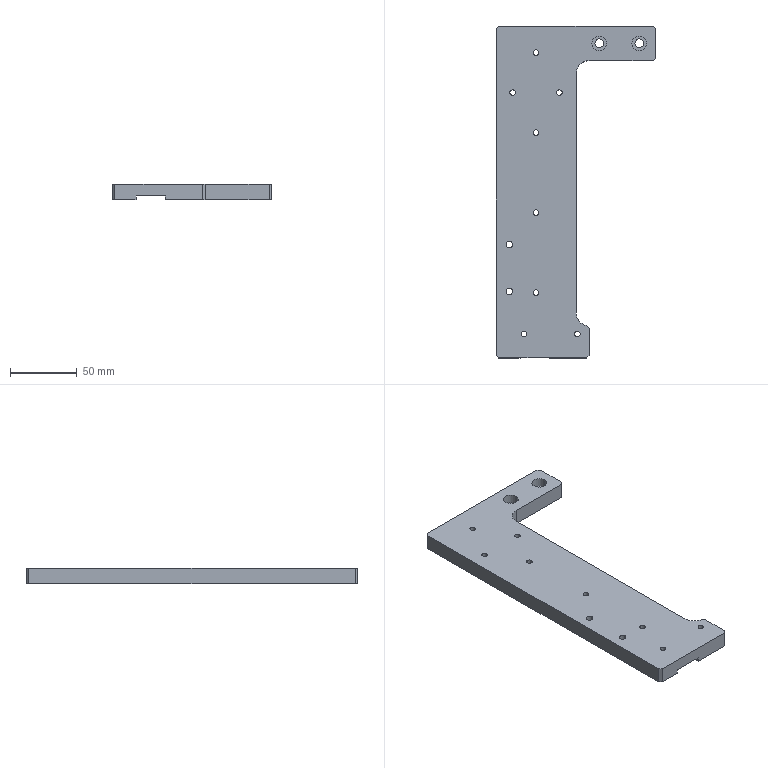Part | SolidWorks | features HoleWzd 5, Chamfer 1, Extrusion 1, ICE 1 | 1 solid | 51 faces | box 120 x 249 x 12 mm | volume 181549 mm3 | cylinder 30 | plane 21 | commonest cylinder face diameters 4.2 x16 5 x4 6.6 x4 11 x4 20 x2